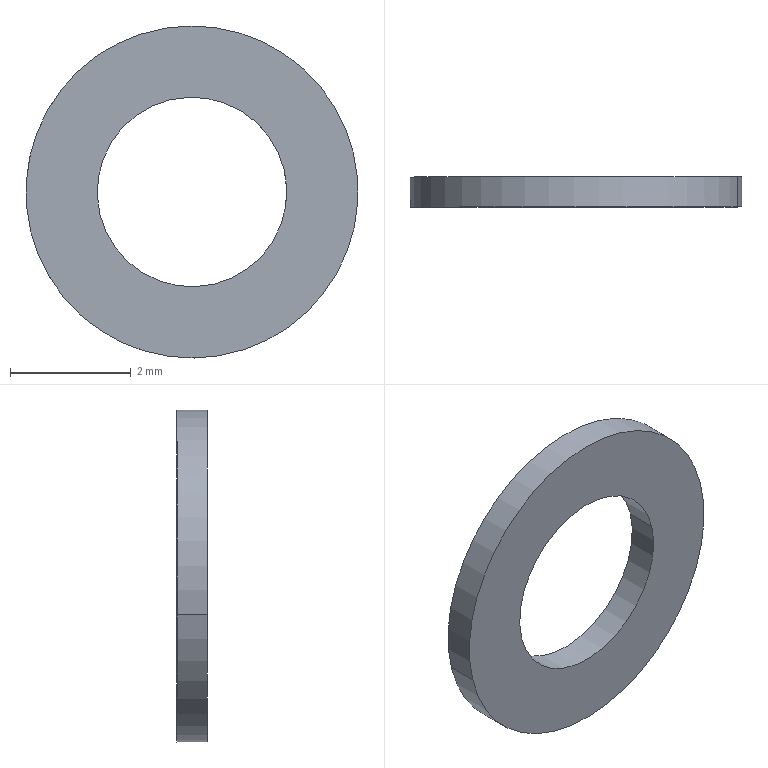Part | SolidWorks | features BaseBody 1 | 1 solid | 6 faces | box 5.5 x 0.5053 x 5.5 mm | volume 8.007 mm3 | cylinder 4 | plane 2 | commonest cylinder face diameters 3.14 x2 5.5 x2
STEP:
#1=CARTESIAN_POINT('',(343.492,378.966,107.288));
#2=VERTEX_POINT('',#1);
#3=CARTESIAN_POINT('',(340.44,378.963,106.551));
#4=VERTEX_POINT('',#3);
#5=CARTESIAN_POINT('',(341.966,378.964,106.919));
#6=DIRECTION('',(0.0009599,-1.,0.));
#7=DIRECTION('',(-0.9721,-0.0009331,-0.2347));
#8=AXIS2_PLACEMENT_3D('',#5,#6,#7);
#9=CIRCLE('',#8,1.57);
#10=EDGE_CURVE('',#2,#4,#9,.T.);
#11=ORIENTED_EDGE('',*,*,#10,.F.);
#12=CARTESIAN_POINT('',(343.493,378.466,107.288));
#13=VERTEX_POINT('',#12);
#14=CARTESIAN_POINT('',(343.492,378.966,107.288));
#15=DIRECTION('',(0.0009599,-1.,0.));
#16=VECTOR('',#15,1000.);
#17=LINE('',#14,#16);
#18=EDGE_CURVE('',#2,#13,#17,.T.);
#19=ORIENTED_EDGE('',*,*,#18,.T.);
#20=CARTESIAN_POINT('',(340.441,378.463,106.551));
#21=VERTEX_POINT('',#20);
#22=CARTESIAN_POINT('',(341.967,378.464,106.919));
#23=DIRECTION('',(-0.0009599,1.,0.));
#24=DIRECTION('',(0.9721,0.0009331,0.2347));
#25=AXIS2_PLACEMENT_3D('',#22,#23,#24);
#26=CIRCLE('',#25,1.57);
#27=EDGE_CURVE('',#21,#13,#26,.T.);
#28=ORIENTED_EDGE('',*,*,#27,.F.);
#29=CARTESIAN_POINT('',(340.44,378.963,106.551));
#30=DIRECTION('',(0.0009599,-1.,0.));
#31=VECTOR('',#30,1000.);
#32=LINE('',#29,#31);
#33=EDGE_CURVE('',#4,#21,#32,.T.);
#34=ORIENTED_EDGE('',*,*,#33,.F.);
#35=EDGE_LOOP('',(#11,#19,#28,#34));
#36=FACE_OUTER_BOUND('',#35,.T.);
#37=CARTESIAN_POINT('',(341.966,378.964,106.919));
#38=DIRECTION('',(0.0009599,-1.,0.));
#39=DIRECTION('',(-0.9721,-0.0009331,-0.2347));
#40=AXIS2_PLACEMENT_3D('',#37,#38,#39);
#41=CYLINDRICAL_SURFACE('',#40,1.57);
#42=ADVANCED_FACE('',(#36),#41,.F.);
#43=CARTESIAN_POINT('',(344.639,378.967,107.564));
#44=VERTEX_POINT('',#43);
#45=CARTESIAN_POINT('',(339.293,378.961,106.274));
#46=VERTEX_POINT('',#45);
#47=CARTESIAN_POINT('',(341.966,378.964,106.919));
#48=DIRECTION('',(-0.0009599,1.,0.));
#49=DIRECTION('',(0.9721,0.0009331,0.2347));
#50=AXIS2_PLACEMENT_3D('',#47,#48,#49);
#51=CIRCLE('',#50,2.75);
#52=EDGE_CURVE('',#44,#46,#51,.T.);
#53=ORIENTED_EDGE('',*,*,#52,.F.);
#54=CARTESIAN_POINT('',(344.64,378.467,107.564));
#55=VERTEX_POINT('',#54);
#56=CARTESIAN_POINT('',(344.639,378.967,107.564));
#57=DIRECTION('',(0.0009599,-1.,0.));
#58=VECTOR('',#57,1000.);
#59=LINE('',#56,#58);
#60=EDGE_CURVE('',#44,#55,#59,.T.);
#61=ORIENTED_EDGE('',*,*,#60,.T.);
#62=CARTESIAN_POINT('',(339.293,378.461,106.274));
#63=VERTEX_POINT('',#62);
#64=CARTESIAN_POINT('',(341.967,378.464,106.919));
#65=DIRECTION('',(0.0009599,-1.,0.));
#66=DIRECTION('',(0.9721,0.0009331,0.2347));
#67=AXIS2_PLACEMENT_3D('',#64,#65,#66);
#68=CIRCLE('',#67,2.75);
#69=EDGE_CURVE('',#63,#55,#68,.T.);
#70=ORIENTED_EDGE('',*,*,#69,.F.);
#71=CARTESIAN_POINT('',(339.293,378.961,106.274));
#72=DIRECTION('',(0.0009599,-1.,0.));
#73=VECTOR('',#72,1000.);
#74=LINE('',#71,#73);
#75=EDGE_CURVE('',#46,#63,#74,.T.);
#76=ORIENTED_EDGE('',*,*,#75,.F.);
#77=EDGE_LOOP('',(#53,#61,#70,#76));
#78=FACE_OUTER_BOUND('',#77,.T.);
#79=CARTESIAN_POINT('',(341.966,378.964,106.919));
#80=DIRECTION('',(0.0009599,-1.,0.));
#81=DIRECTION('',(-0.9721,-0.0009331,-0.2347));
#82=AXIS2_PLACEMENT_3D('',#79,#80,#81);
#83=CYLINDRICAL_SURFACE('',#82,2.75);
#84=ADVANCED_FACE('',(#78),#83,.T.);
#85=ORIENTED_EDGE('',*,*,#27,.T.);
#86=CARTESIAN_POINT('',(341.967,378.464,106.919));
#87=DIRECTION('',(-0.0009599,1.,0.));
#88=DIRECTION('',(0.9721,0.0009331,0.2347));
#89=AXIS2_PLACEMENT_3D('',#86,#87,#88);
#90=CIRCLE('',#89,1.57);
#91=EDGE_CURVE('',#13,#21,#90,.T.);
#92=ORIENTED_EDGE('',*,*,#91,.T.);
#93=EDGE_LOOP('',(#85,#92));
#94=FACE_BOUND('',#93,.T.);
#95=ORIENTED_EDGE('',*,*,#69,.T.);
#96=CARTESIAN_POINT('',(341.967,378.464,106.919));
#97=DIRECTION('',(0.0009599,-1.,0.));
#98=DIRECTION('',(0.9721,0.0009331,0.2347));
#99=AXIS2_PLACEMENT_3D('',#96,#97,#98);
#100=CIRCLE('',#99,2.75);
#101=EDGE_CURVE('',#55,#63,#100,.T.);
#102=ORIENTED_EDGE('',*,*,#101,.T.);
#103=EDGE_LOOP('',(#95,#102));
#104=FACE_OUTER_BOUND('',#103,.T.);
#105=CARTESIAN_POINT('',(341.967,378.464,106.919));
#106=DIRECTION('',(-0.0009599,1.,0.));
#107=DIRECTION('',(0.,0.,1.));
#108=AXIS2_PLACEMENT_3D('',#105,#106,#107);
#109=PLANE('',#108);
#110=ADVANCED_FACE('',(#94,#104),#109,.F.);
#111=ORIENTED_EDGE('',*,*,#60,.F.);
#112=CARTESIAN_POINT('',(341.966,378.964,106.919));
#113=DIRECTION('',(-0.0009599,1.,0.));
#114=DIRECTION('',(0.9721,0.0009331,0.2347));
#115=AXIS2_PLACEMENT_3D('',#112,#113,#114);
#116=CIRCLE('',#115,2.75);
#117=EDGE_CURVE('',#46,#44,#116,.T.);
#118=ORIENTED_EDGE('',*,*,#117,.F.);
#119=ORIENTED_EDGE('',*,*,#75,.T.);
#120=ORIENTED_EDGE('',*,*,#101,.F.);
#121=EDGE_LOOP('',(#111,#118,#119,#120));
#122=FACE_OUTER_BOUND('',#121,.T.);
#123=CARTESIAN_POINT('',(341.966,378.964,106.919));
#124=DIRECTION('',(0.0009599,-1.,0.));
#125=DIRECTION('',(-0.9721,-0.0009331,-0.2347));
#126=AXIS2_PLACEMENT_3D('',#123,#124,#125);
#127=CYLINDRICAL_SURFACE('',#126,2.75);
#128=ADVANCED_FACE('',(#122),#127,.T.);
#129=CARTESIAN_POINT('',(341.966,378.964,106.919));
#130=DIRECTION('',(0.0009599,-1.,0.));
#131=DIRECTION('',(-0.9721,-0.0009331,-0.2347));
#132=AXIS2_PLACEMENT_3D('',#129,#130,#131);
#133=CIRCLE('',#132,1.57);
#134=EDGE_CURVE('',#4,#2,#133,.T.);
#135=ORIENTED_EDGE('',*,*,#134,.T.);
#136=ORIENTED_EDGE('',*,*,#10,.T.);
#137=EDGE_LOOP('',(#135,#136));
#138=FACE_BOUND('',#137,.T.);
#139=ORIENTED_EDGE('',*,*,#117,.T.);
#140=ORIENTED_EDGE('',*,*,#52,.T.);
#141=EDGE_LOOP('',(#139,#140));
#142=FACE_OUTER_BOUND('',#141,.T.);
#143=CARTESIAN_POINT('',(341.966,378.964,106.919));
#144=DIRECTION('',(-0.0009599,1.,0.));
#145=DIRECTION('',(0.,0.,1.));
#146=AXIS2_PLACEMENT_3D('',#143,#144,#145);
#147=PLANE('',#146);
#148=ADVANCED_FACE('',(#138,#142),#147,.T.);
#149=ORIENTED_EDGE('',*,*,#18,.F.);
#150=ORIENTED_EDGE('',*,*,#134,.F.);
#151=ORIENTED_EDGE('',*,*,#33,.T.);
#152=ORIENTED_EDGE('',*,*,#91,.F.);
#153=EDGE_LOOP('',(#149,#150,#151,#152));
#154=FACE_OUTER_BOUND('',#153,.T.);
#155=CARTESIAN_POINT('',(341.966,378.964,106.919));
#156=DIRECTION('',(0.0009599,-1.,0.));
#157=DIRECTION('',(-0.9721,-0.0009331,-0.2347));
#158=AXIS2_PLACEMENT_3D('',#155,#156,#157);
#159=CYLINDRICAL_SURFACE('',#158,1.57);
#160=ADVANCED_FACE('',(#154),#159,.F.);
#161=CLOSED_SHELL('',(#42,#84,#110,#128,#148,#160));
#162=MANIFOLD_SOLID_BREP('',#161);
#163=CARTESIAN_POINT('',(0.,0.,0.));
#164=DIRECTION('',(0.,0.,1.));
#165=DIRECTION('',(1.,0.,0.));
#166=AXIS2_PLACEMENT_3D('',#163,#164,#165);
#167=(LENGTH_UNIT()NAMED_UNIT(*)SI_UNIT(.MILLI.,.METRE.));
#168=UNCERTAINTY_MEASURE_WITH_UNIT(LENGTH_MEASURE(0.00001),#167,'','');
#169=(NAMED_UNIT(*)PLANE_ANGLE_UNIT()SI_UNIT($,.RADIAN.));
#170=(NAMED_UNIT(*)SI_UNIT($,.STERADIAN.)SOLID_ANGLE_UNIT());
#171=(GEOMETRIC_REPRESENTATION_CONTEXT(3)GLOBAL_UNCERTAINTY_ASSIGNED_CONTEXT((#168))GLOBAL_UNIT_ASSIGNED_CONTEXT((#167,#169,#170))REPRESENTATION_CONTEXT('',''));
#172=ADVANCED_BREP_SHAPE_REPRESENTATION('',(#162,#166),#171);